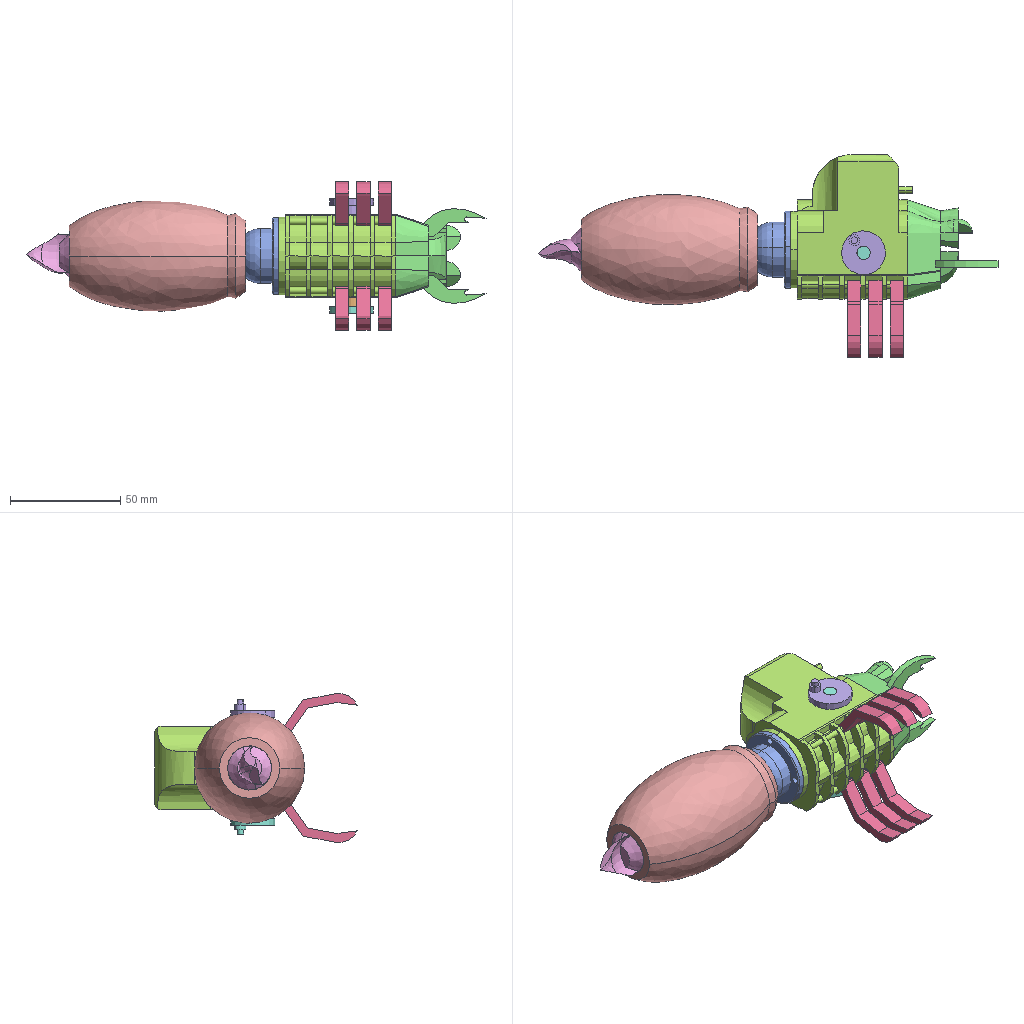Assembly | SolidWorks | 9 different items | 14 placed | box 208 x 92 x 67 mm
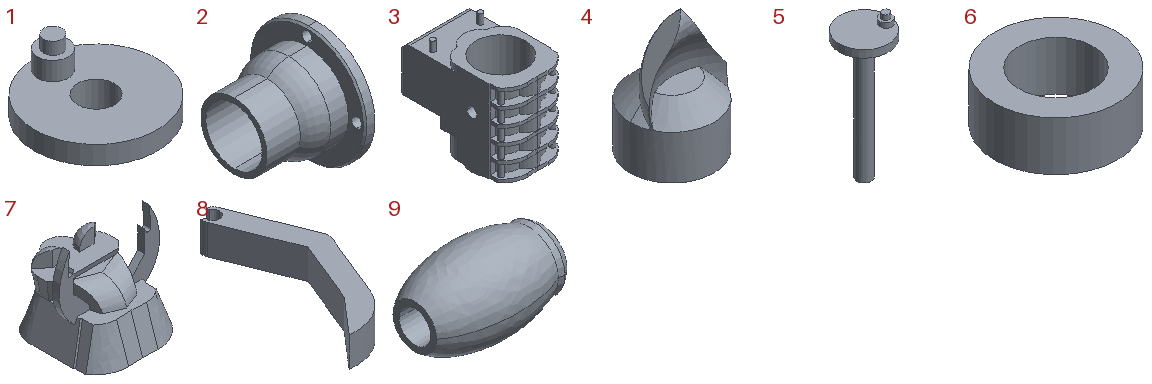Parts list (item | quantity | size | volume | features):
1 | x1 | 20 x 20 x 12 mm | 1012 mm3 | features ICE 5, Extrusion 1
2 | x1 | 25 x 35 x 35 mm | 5761 mm3 | features ICE 3, Chamfer 1, Extrusion 1, Fillet 1
3 | x1 | 37.876 x 65.524 x 55.021 mm | 67131 mm3 | features ICE 12, Cut 6, Fillet 4, Chamfer 2, MirrorPattern 2, Extrusion 1, LPattern 1
4 | x1 | 20 x 20 x 30.002 mm | 4792 mm3 | features ICE 3, Chamfer 1, Extrusion 1, Fillet 1, Sweep 1
5 | x1 | 20 x 20 x 55.88 mm | 2378 mm3 | features ICE 5, Extrusion 1
6 | x1 | 10 x 10 x 4 mm | 201.062 mm3 | features Extrusion 1
7 | x1 | 43.024 x 45 x 40.937 mm | 22847 mm3 | features ICE 3, MirrorPattern 3, Blend 1, Cut 1, Fillet 1, Revolution 1
8 | x6 | 15.303 x 36.626 x 6 mm | 919.383 mm3 | features Extrusion 1
9 | x1 | 80 x 50 x 50 mm | 97007 mm3 | features Chamfer 1, ICE 1, Revolution 1
Mates (type | each side: item.copy, entity, surface, feature):
Concentric | 9.1 face cylinder Revolve2 | 2.1 face cylinder Boss-Extrude1
Coincident | 9.1 face plane Revolve2 | 2.1 edge
Concentric | 2.1 face cylinder Boss-Extrude1 | 3.1 face cylinder Cut-Extrude2
Coincident | 2.1 face plane Boss-Extrude2 | 3.1 face plane Boss-Extrude1
Concentric | 9.1 face cylinder Revolve2 | 4.1 face cylinder Boss-Extrude1
Coincident | 9.1 edge | 4.1 edge
Concentric | 3.1 face cylinder Cut-Extrude3 | 5.1 face cylinder Boss-Extrude4
Coincident | 3.1 plane | assembly plane
Concentric | 5.1 face cylinder Boss-Extrude4 | 6.1 face cylinder Boss-Extrude1
Coincident | 3.1 face plane Mirror1 | 6.1 face plane Boss-Extrude1
Coincident | 5.1 face plane Boss-Extrude1 | 6.1 face plane Boss-Extrude1
Concentric | 5.1 face cylinder Boss-Extrude3 | assembly face
Coincident | 5.1 face plane Boss-Extrude3 | assembly face
Concentric | assembly face | assembly face | 5 times
Coincident | assembly face | assembly face | 5 times
Coincident | 3.1 face plane Mirror1 | assembly face
Parallel | 3.1 face plane Boss-Extrude6 | assembly face
Width | assembly face | assembly face | 3.1 face plane Boss-Extrude6 | 3.1 face plane Boss-Extrude6
Concentric | 5.1 face cylinder Boss-Extrude4 | 1.1 face cylinder Cut-Extrude1
Coincident | 3.1 face plane Boss-Extrude5 | 1.1 face plane Boss-Extrude4
Concentric | 3.1 face cylinder Cut-Extrude5 | assembly face
Concentric | 3.1 face cylinder Boss-Extrude8 | assembly face
InPlace | 3.1 face plane Boss-Extrude2 | 7.1 plane
Concentric | 3.1 face cylinder Boss-Extrude12 | 8.1 face cylinder Boss-Extrude1
Coincident | 3.1 face plane Boss-Extrude10 | 8.1 face plane Boss-Extrude1
Concentric | 2.1 face cylinder Boss-Extrude1 | assembly face
Concentric | 5.1 face cylinder Boss-Extrude4 | assembly face
GearDim | assembly face | assembly face
DistanceDim | 6.1 face plane Boss-Extrude1 | assembly face
DistanceDim | assembly face | 2.1 face plane Boss-Extrude2
Coincident | 1.1 plane | assembly plane